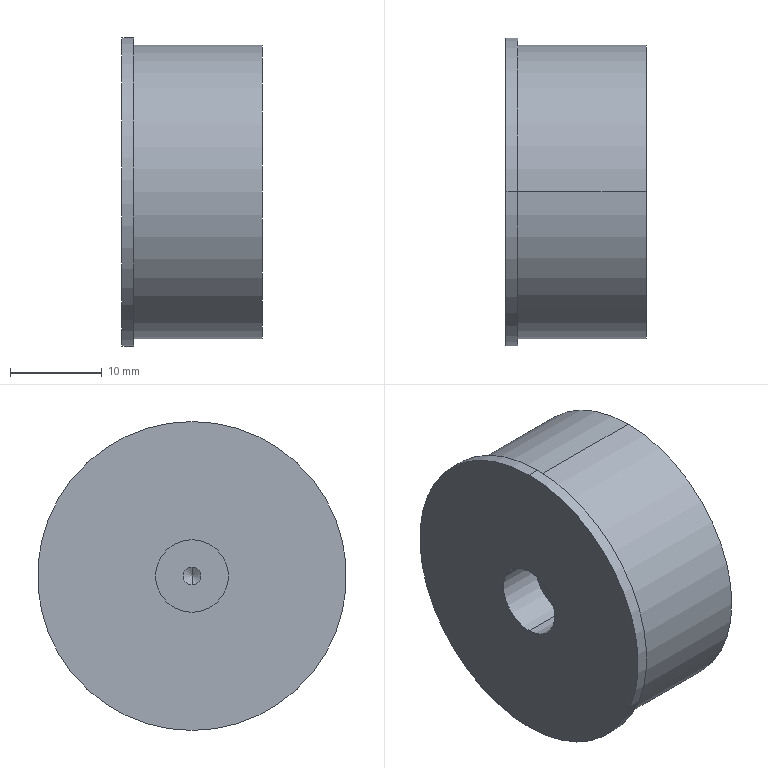Part | SolidWorks | features BaseBody 1 | 1 solid | 12 faces | box 15.3 x 33.7 x 33.7 mm | volume 12172 mm3 | cylinder 6 | plane 4 | cone 2 | commonest cylinder face diameters 7.928 x2 32 x2 33.7 x2
STEP:
#1=CARTESIAN_POINT('',(209.5,-84.,116.471));
#2=VERTEX_POINT('',#1);
#3=CARTESIAN_POINT('',(209.5,-84.,82.771));
#4=VERTEX_POINT('',#3);
#5=CARTESIAN_POINT('',(209.5,-84.,99.621));
#6=DIRECTION('',(-1.,0.,0.));
#7=DIRECTION('',(0.,0.,1.));
#8=AXIS2_PLACEMENT_3D('',#5,#6,#7);
#9=CIRCLE('',#8,16.85);
#10=EDGE_CURVE('',#2,#4,#9,.T.);
#11=ORIENTED_EDGE('',*,*,#10,.T.);
#12=CARTESIAN_POINT('',(208.2,-84.,82.771));
#13=VERTEX_POINT('',#12);
#14=CARTESIAN_POINT('',(209.5,-84.,82.771));
#15=DIRECTION('',(-1.,0.,0.));
#16=VECTOR('',#15,1000.);
#17=LINE('',#14,#16);
#18=EDGE_CURVE('',#4,#13,#17,.T.);
#19=ORIENTED_EDGE('',*,*,#18,.T.);
#20=CARTESIAN_POINT('',(208.2,-84.,116.471));
#21=VERTEX_POINT('',#20);
#22=CARTESIAN_POINT('',(208.2,-84.,99.621));
#23=DIRECTION('',(1.,0.,0.));
#24=DIRECTION('',(0.,0.,1.));
#25=AXIS2_PLACEMENT_3D('',#22,#23,#24);
#26=CIRCLE('',#25,16.85);
#27=EDGE_CURVE('',#13,#21,#26,.T.);
#28=ORIENTED_EDGE('',*,*,#27,.T.);
#29=CARTESIAN_POINT('',(209.5,-84.,116.471));
#30=DIRECTION('',(-1.,0.,0.));
#31=VECTOR('',#30,1000.);
#32=LINE('',#29,#31);
#33=EDGE_CURVE('',#2,#21,#32,.T.);
#34=ORIENTED_EDGE('',*,*,#33,.F.);
#35=EDGE_LOOP('',(#11,#19,#28,#34));
#36=FACE_OUTER_BOUND('',#35,.T.);
#37=CARTESIAN_POINT('',(209.5,-84.,99.621));
#38=DIRECTION('',(-1.,0.,0.));
#39=DIRECTION('',(0.,0.,1.));
#40=AXIS2_PLACEMENT_3D('',#37,#38,#39);
#41=CYLINDRICAL_SURFACE('',#40,16.85);
#42=ADVANCED_FACE('',(#36),#41,.T.);
#43=CARTESIAN_POINT('',(213.2,-84.,95.657));
#44=VERTEX_POINT('',#43);
#45=CARTESIAN_POINT('',(213.2,-84.,103.585));
#46=VERTEX_POINT('',#45);
#47=CARTESIAN_POINT('',(213.2,-84.,99.621));
#48=DIRECTION('',(-1.,0.,0.));
#49=DIRECTION('',(0.,0.,1.));
#50=AXIS2_PLACEMENT_3D('',#47,#48,#49);
#51=CIRCLE('',#50,3.964);
#52=EDGE_CURVE('',#44,#46,#51,.T.);
#53=ORIENTED_EDGE('',*,*,#52,.F.);
#54=CARTESIAN_POINT('',(208.2,-84.,95.657));
#55=VERTEX_POINT('',#54);
#56=CARTESIAN_POINT('',(213.2,-84.,95.657));
#57=DIRECTION('',(-1.,0.,0.));
#58=VECTOR('',#57,1000.);
#59=LINE('',#56,#58);
#60=EDGE_CURVE('',#44,#55,#59,.T.);
#61=ORIENTED_EDGE('',*,*,#60,.T.);
#62=CARTESIAN_POINT('',(208.2,-84.,103.585));
#63=VERTEX_POINT('',#62);
#64=CARTESIAN_POINT('',(208.2,-84.,99.621));
#65=DIRECTION('',(-1.,0.,0.));
#66=DIRECTION('',(0.,0.,1.));
#67=AXIS2_PLACEMENT_3D('',#64,#65,#66);
#68=CIRCLE('',#67,3.964);
#69=EDGE_CURVE('',#55,#63,#68,.T.);
#70=ORIENTED_EDGE('',*,*,#69,.T.);
#71=CARTESIAN_POINT('',(213.2,-84.,103.585));
#72=DIRECTION('',(-1.,0.,0.));
#73=VECTOR('',#72,1000.);
#74=LINE('',#71,#73);
#75=EDGE_CURVE('',#46,#63,#74,.T.);
#76=ORIENTED_EDGE('',*,*,#75,.F.);
#77=EDGE_LOOP('',(#53,#61,#70,#76));
#78=FACE_OUTER_BOUND('',#77,.T.);
#79=CARTESIAN_POINT('',(213.2,-84.,99.621));
#80=DIRECTION('',(-1.,0.,0.));
#81=DIRECTION('',(0.,0.,1.));
#82=AXIS2_PLACEMENT_3D('',#79,#80,#81);
#83=CYLINDRICAL_SURFACE('',#82,3.964);
#84=ADVANCED_FACE('',(#78),#83,.F.);
#85=CARTESIAN_POINT('',(223.5,-84.,115.621));
#86=VERTEX_POINT('',#85);
#87=CARTESIAN_POINT('',(223.5,-84.,83.621));
#88=VERTEX_POINT('',#87);
#89=CARTESIAN_POINT('',(223.5,-84.,99.621));
#90=DIRECTION('',(-1.,0.,0.));
#91=DIRECTION('',(0.,0.,1.));
#92=AXIS2_PLACEMENT_3D('',#89,#90,#91);
#93=CIRCLE('',#92,16.);
#94=EDGE_CURVE('',#86,#88,#93,.T.);
#95=ORIENTED_EDGE('',*,*,#94,.T.);
#96=CARTESIAN_POINT('',(209.5,-84.,83.621));
#97=VERTEX_POINT('',#96);
#98=CARTESIAN_POINT('',(223.5,-84.,83.621));
#99=DIRECTION('',(-1.,0.,0.));
#100=VECTOR('',#99,1000.);
#101=LINE('',#98,#100);
#102=EDGE_CURVE('',#88,#97,#101,.T.);
#103=ORIENTED_EDGE('',*,*,#102,.T.);
#104=CARTESIAN_POINT('',(209.5,-84.,115.621));
#105=VERTEX_POINT('',#104);
#106=CARTESIAN_POINT('',(209.5,-84.,99.621));
#107=DIRECTION('',(-1.,0.,0.));
#108=DIRECTION('',(0.,0.,1.));
#109=AXIS2_PLACEMENT_3D('',#106,#107,#108);
#110=CIRCLE('',#109,16.);
#111=EDGE_CURVE('',#105,#97,#110,.T.);
#112=ORIENTED_EDGE('',*,*,#111,.F.);
#113=CARTESIAN_POINT('',(223.5,-84.,115.621));
#114=DIRECTION('',(-1.,0.,0.));
#115=VECTOR('',#114,1000.);
#116=LINE('',#113,#115);
#117=EDGE_CURVE('',#86,#105,#116,.T.);
#118=ORIENTED_EDGE('',*,*,#117,.F.);
#119=EDGE_LOOP('',(#95,#103,#112,#118));
#120=FACE_OUTER_BOUND('',#119,.T.);
#121=CARTESIAN_POINT('',(223.5,-84.,99.621));
#122=DIRECTION('',(-1.,0.,0.));
#123=DIRECTION('',(0.,0.,1.));
#124=AXIS2_PLACEMENT_3D('',#121,#122,#123);
#125=CYLINDRICAL_SURFACE('',#124,16.);
#126=ADVANCED_FACE('',(#120),#125,.T.);
#127=CARTESIAN_POINT('',(213.782,-84.,99.621));
#128=VERTEX_POINT('',#127);
#129=CARTESIAN_POINT('',(213.2,-84.,100.59));
#130=VERTEX_POINT('',#129);
#131=CARTESIAN_POINT('',(213.2,-84.,100.59));
#132=DIRECTION('',(-0.515,0.,0.8572));
#133=VECTOR('',#132,1000.);
#134=LINE('',#131,#133);
#135=EDGE_CURVE('',#128,#130,#134,.T.);
#136=ORIENTED_EDGE('',*,*,#135,.F.);
#137=CARTESIAN_POINT('',(213.2,-84.,98.653));
#138=VERTEX_POINT('',#137);
#139=CARTESIAN_POINT('',(213.2,-84.,98.653));
#140=DIRECTION('',(-0.515,0.,-0.8572));
#141=VECTOR('',#140,1000.);
#142=LINE('',#139,#141);
#143=EDGE_CURVE('',#128,#138,#142,.T.);
#144=ORIENTED_EDGE('',*,*,#143,.T.);
#145=CARTESIAN_POINT('',(213.2,-84.,99.621));
#146=DIRECTION('',(1.,0.,0.));
#147=DIRECTION('',(0.,0.,1.));
#148=AXIS2_PLACEMENT_3D('',#145,#146,#147);
#149=CIRCLE('',#148,0.9685);
#150=EDGE_CURVE('',#130,#138,#149,.T.);
#151=ORIENTED_EDGE('',*,*,#150,.F.);
#152=EDGE_LOOP('',(#136,#144,#151));
#153=FACE_OUTER_BOUND('',#152,.T.);
#154=CARTESIAN_POINT('',(213.2,-84.,99.621));
#155=DIRECTION('',(-1.,0.,0.));
#156=DIRECTION('',(0.,0.,1.));
#157=AXIS2_PLACEMENT_3D('',#154,#155,#156);
#158=CONICAL_SURFACE('',#157,0.9685,1.03);
#159=ADVANCED_FACE('',(#153),#158,.F.);
#160=CARTESIAN_POINT('',(208.2,-84.,99.621));
#161=DIRECTION('',(1.,0.,0.));
#162=DIRECTION('',(0.,0.,1.));
#163=AXIS2_PLACEMENT_3D('',#160,#161,#162);
#164=CIRCLE('',#163,16.85);
#165=EDGE_CURVE('',#21,#13,#164,.T.);
#166=ORIENTED_EDGE('',*,*,#165,.F.);
#167=ORIENTED_EDGE('',*,*,#27,.F.);
#168=EDGE_LOOP('',(#166,#167));
#169=FACE_OUTER_BOUND('',#168,.T.);
#170=CARTESIAN_POINT('',(208.2,-84.,99.621));
#171=DIRECTION('',(-1.,0.,0.));
#172=DIRECTION('',(0.,0.,1.));
#173=AXIS2_PLACEMENT_3D('',#170,#171,#172);
#174=CIRCLE('',#173,3.964);
#175=EDGE_CURVE('',#63,#55,#174,.T.);
#176=ORIENTED_EDGE('',*,*,#175,.F.);
#177=ORIENTED_EDGE('',*,*,#69,.F.);
#178=EDGE_LOOP('',(#176,#177));
#179=FACE_BOUND('',#178,.T.);
#180=CARTESIAN_POINT('',(208.2,-84.,99.621));
#181=DIRECTION('',(1.,0.,0.));
#182=DIRECTION('',(0.,0.,-1.));
#183=AXIS2_PLACEMENT_3D('',#180,#181,#182);
#184=PLANE('',#183);
#185=ADVANCED_FACE('',(#169,#179),#184,.F.);
#186=ORIENTED_EDGE('',*,*,#18,.F.);
#187=CARTESIAN_POINT('',(209.5,-84.,99.621));
#188=DIRECTION('',(-1.,0.,0.));
#189=DIRECTION('',(0.,0.,1.));
#190=AXIS2_PLACEMENT_3D('',#187,#188,#189);
#191=CIRCLE('',#190,16.85);
#192=EDGE_CURVE('',#4,#2,#191,.T.);
#193=ORIENTED_EDGE('',*,*,#192,.T.);
#194=ORIENTED_EDGE('',*,*,#33,.T.);
#195=ORIENTED_EDGE('',*,*,#165,.T.);
#196=EDGE_LOOP('',(#186,#193,#194,#195));
#197=FACE_OUTER_BOUND('',#196,.T.);
#198=CARTESIAN_POINT('',(209.5,-84.,99.621));
#199=DIRECTION('',(-1.,0.,0.));
#200=DIRECTION('',(0.,0.,1.));
#201=AXIS2_PLACEMENT_3D('',#198,#199,#200);
#202=CYLINDRICAL_SURFACE('',#201,16.85);
#203=ADVANCED_FACE('',(#197),#202,.T.);
#204=ORIENTED_EDGE('',*,*,#60,.F.);
#205=CARTESIAN_POINT('',(213.2,-84.,99.621));
#206=DIRECTION('',(-1.,0.,0.));
#207=DIRECTION('',(0.,0.,1.));
#208=AXIS2_PLACEMENT_3D('',#205,#206,#207);
#209=CIRCLE('',#208,3.964);
#210=EDGE_CURVE('',#46,#44,#209,.T.);
#211=ORIENTED_EDGE('',*,*,#210,.F.);
#212=ORIENTED_EDGE('',*,*,#75,.T.);
#213=ORIENTED_EDGE('',*,*,#175,.T.);
#214=EDGE_LOOP('',(#204,#211,#212,#213));
#215=FACE_OUTER_BOUND('',#214,.T.);
#216=CARTESIAN_POINT('',(213.2,-84.,99.621));
#217=DIRECTION('',(-1.,0.,0.));
#218=DIRECTION('',(0.,0.,1.));
#219=AXIS2_PLACEMENT_3D('',#216,#217,#218);
#220=CYLINDRICAL_SURFACE('',#219,3.964);
#221=ADVANCED_FACE('',(#215),#220,.F.);
#222=ORIENTED_EDGE('',*,*,#111,.T.);
#223=CARTESIAN_POINT('',(209.5,-84.,99.621));
#224=DIRECTION('',(-1.,0.,0.));
#225=DIRECTION('',(0.,0.,1.));
#226=AXIS2_PLACEMENT_3D('',#223,#224,#225);
#227=CIRCLE('',#226,16.);
#228=EDGE_CURVE('',#97,#105,#227,.T.);
#229=ORIENTED_EDGE('',*,*,#228,.T.);
#230=EDGE_LOOP('',(#222,#229));
#231=FACE_BOUND('',#230,.T.);
#232=ORIENTED_EDGE('',*,*,#10,.F.);
#233=ORIENTED_EDGE('',*,*,#192,.F.);
#234=EDGE_LOOP('',(#232,#233));
#235=FACE_OUTER_BOUND('',#234,.T.);
#236=CARTESIAN_POINT('',(209.5,-84.,99.621));
#237=DIRECTION('',(1.,0.,0.));
#238=DIRECTION('',(0.,0.,-1.));
#239=AXIS2_PLACEMENT_3D('',#236,#237,#238);
#240=PLANE('',#239);
#241=ADVANCED_FACE('',(#231,#235),#240,.T.);
#242=ORIENTED_EDGE('',*,*,#150,.T.);
#243=CARTESIAN_POINT('',(213.2,-84.,99.621));
#244=DIRECTION('',(1.,0.,0.));
#245=DIRECTION('',(0.,0.,1.));
#246=AXIS2_PLACEMENT_3D('',#243,#244,#245);
#247=CIRCLE('',#246,0.9685);
#248=EDGE_CURVE('',#138,#130,#247,.T.);
#249=ORIENTED_EDGE('',*,*,#248,.T.);
#250=EDGE_LOOP('',(#242,#249));
#251=FACE_BOUND('',#250,.T.);
#252=ORIENTED_EDGE('',*,*,#210,.T.);
#253=ORIENTED_EDGE('',*,*,#52,.T.);
#254=EDGE_LOOP('',(#252,#253));
#255=FACE_OUTER_BOUND('',#254,.T.);
#256=CARTESIAN_POINT('',(213.2,-84.,99.621));
#257=DIRECTION('',(-1.,0.,0.));
#258=DIRECTION('',(0.,0.,1.));
#259=AXIS2_PLACEMENT_3D('',#256,#257,#258);
#260=PLANE('',#259);
#261=ADVANCED_FACE('',(#251,#255),#260,.T.);
#262=ORIENTED_EDGE('',*,*,#102,.F.);
#263=CARTESIAN_POINT('',(223.5,-84.,99.621));
#264=DIRECTION('',(-1.,0.,0.));
#265=DIRECTION('',(0.,0.,1.));
#266=AXIS2_PLACEMENT_3D('',#263,#264,#265);
#267=CIRCLE('',#266,16.);
#268=EDGE_CURVE('',#88,#86,#267,.T.);
#269=ORIENTED_EDGE('',*,*,#268,.T.);
#270=ORIENTED_EDGE('',*,*,#117,.T.);
#271=ORIENTED_EDGE('',*,*,#228,.F.);
#272=EDGE_LOOP('',(#262,#269,#270,#271));
#273=FACE_OUTER_BOUND('',#272,.T.);
#274=CARTESIAN_POINT('',(223.5,-84.,99.621));
#275=DIRECTION('',(-1.,0.,0.));
#276=DIRECTION('',(0.,0.,1.));
#277=AXIS2_PLACEMENT_3D('',#274,#275,#276);
#278=CYLINDRICAL_SURFACE('',#277,16.);
#279=ADVANCED_FACE('',(#273),#278,.T.);
#280=ORIENTED_EDGE('',*,*,#143,.F.);
#281=ORIENTED_EDGE('',*,*,#135,.T.);
#282=ORIENTED_EDGE('',*,*,#248,.F.);
#283=EDGE_LOOP('',(#280,#281,#282));
#284=FACE_OUTER_BOUND('',#283,.T.);
#285=CARTESIAN_POINT('',(213.2,-84.,99.621));
#286=DIRECTION('',(-1.,0.,0.));
#287=DIRECTION('',(0.,0.,1.));
#288=AXIS2_PLACEMENT_3D('',#285,#286,#287);
#289=CONICAL_SURFACE('',#288,0.9685,1.03);
#290=ADVANCED_FACE('',(#284),#289,.F.);
#291=ORIENTED_EDGE('',*,*,#94,.F.);
#292=ORIENTED_EDGE('',*,*,#268,.F.);
#293=EDGE_LOOP('',(#291,#292));
#294=FACE_OUTER_BOUND('',#293,.T.);
#295=CARTESIAN_POINT('',(223.5,-84.,99.621));
#296=DIRECTION('',(1.,0.,0.));
#297=DIRECTION('',(0.,0.,-1.));
#298=AXIS2_PLACEMENT_3D('',#295,#296,#297);
#299=PLANE('',#298);
#300=ADVANCED_FACE('',(#294),#299,.T.);
#301=CLOSED_SHELL('',(#42,#84,#126,#159,#185,#203,#221,#241,#261,#279,#290,#300));
#302=MANIFOLD_SOLID_BREP('',#301);
#303=CARTESIAN_POINT('',(0.,0.,0.));
#304=DIRECTION('',(0.,0.,1.));
#305=DIRECTION('',(1.,0.,0.));
#306=AXIS2_PLACEMENT_3D('',#303,#304,#305);
#307=(LENGTH_UNIT()NAMED_UNIT(*)SI_UNIT(.MILLI.,.METRE.));
#308=UNCERTAINTY_MEASURE_WITH_UNIT(LENGTH_MEASURE(0.00001),#307,'','');
#309=(NAMED_UNIT(*)PLANE_ANGLE_UNIT()SI_UNIT($,.RADIAN.));
#310=(NAMED_UNIT(*)SI_UNIT($,.STERADIAN.)SOLID_ANGLE_UNIT());
#311=(GEOMETRIC_REPRESENTATION_CONTEXT(3)GLOBAL_UNCERTAINTY_ASSIGNED_CONTEXT((#308))GLOBAL_UNIT_ASSIGNED_CONTEXT((#307,#309,#310))REPRESENTATION_CONTEXT('',''));
#312=ADVANCED_BREP_SHAPE_REPRESENTATION('',(#302,#306),#311);